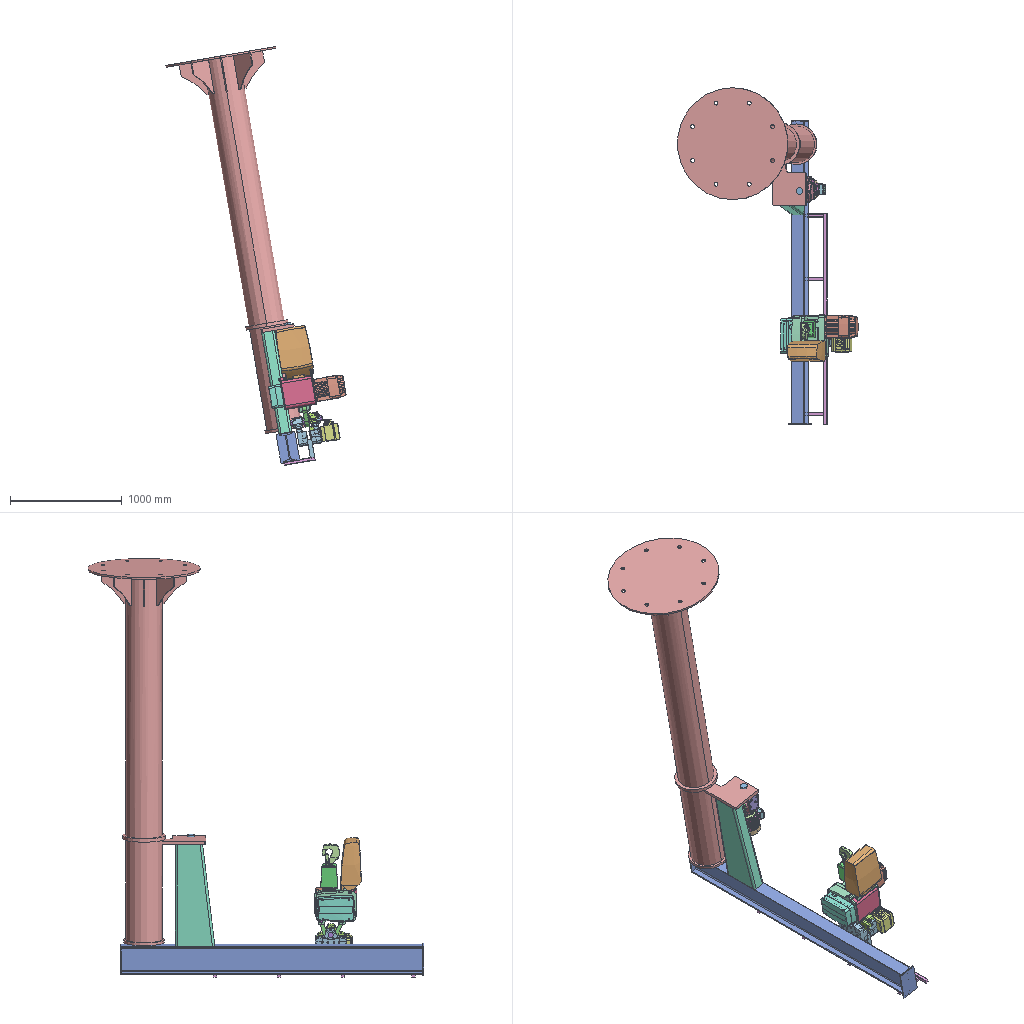Assembly | SolidWorks | 18 different items | 18 placed | box 1611 x 3000 x 3741 mm
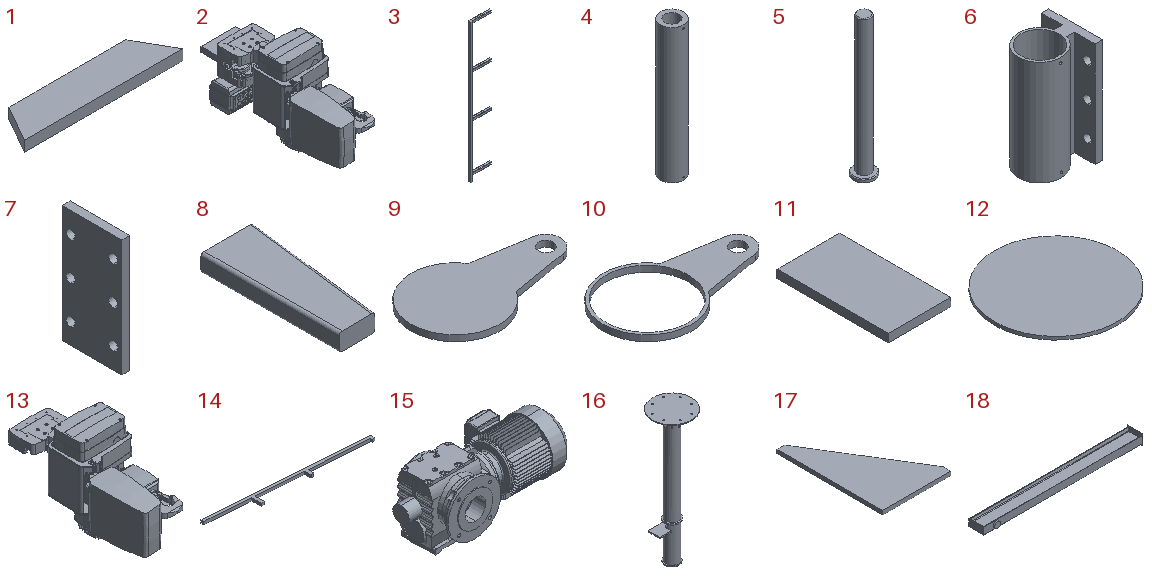Parts list (item | quantity | size | volume | features):
1 | x1 | 152 x 35 x 10 mm | 46200 mm3 | features Extrusion 1
2 | x1 | - | 83796810 mm3 | features BaseBody 21, ICE 3, Scale 1
3 | x1 | 280 x 30 x 1880 mm | 2561715 mm3 | features Extrusion 1, ICE 1
4 | x1 | 80 x 80 x 470 mm | 1439045 mm3 | features Extrusion 1, ICE 1
5 | x1 | 82 x 82 x 541 mm | 1109073 mm3 | features Chamfer 1, Extrusion 1, ICE 1
6 | x1 | 120 x 112 x 220 mm | 732141 mm3 | features ICE 2, Extrusion 1
7 | x1 | 15 x 112 x 220 mm | 349172 mm3 | features ICE 3, Extrusion 1
8 | x1 | 350 x 923 x 118 mm | 31811585 mm3 | features Extrusion 1, Fillet 1
9 | x1 | 496.5 x 293 x 20 mm | 1799574 mm3 | features Extrusion 1
10 | x1 | 496.5 x 293 x 20 mm | 628876 mm3 | features Extrusion 1
11 | x1 | 152 x 270 x 20 mm | 820800 mm3 | features Extrusion 1
12 | x1 | 760 x 760 x 20 mm | 9072920 mm3 | features Extrusion 1
13 | x1 | 284.321 x 725.83 x 459.6 mm | 19917638 mm3 | features BaseBody 17, Scale 1
14 | x1 | 2200 x 220 x 40 mm | 3909881 mm3 | features Extrusion 1
15 | x1 | 558 x 283.5 x 240 mm | 14328030 mm3 | features BaseBody 18, ICE 2
16 | x1 | 1050 x 1000 x 3392 mm | 86673581 mm3 | features ICE 6, CirPattern 1, Extrusion 1
17 | x1 | 180 x 280 x 10 mm | 296000 mm3 | features Extrusion 1
18 | x1 | 2710 x 284 x 170 mm | 14871084 mm3 | features ICE 3, Fillet 2, Extrusion 1
Mates (type | each side: item.copy, entity, surface, feature):
Concentric | 16.1 face cylinder Boss-Extrude1 | 18.1 face cylinder Boss-Extrude3
Coincident | 16.1 face plane Boss-Extrude5 | 18.1 face plane Boss-Extrude3
Parallel | 18.1 face plane Boss-Extrude2 | assembly plane
DistanceDim | 2.1 vertex | 16.1 face plane Boss-Extrude3
Coincident | 18.1 face plane Base | 3.1 face plane Boss-Extrude2 | 2 times
Coincident | 18.1 face plane Boss-Extrude2 | 3.1 face plane Boss-Extrude1
Coincident | 2.1 face plane Boss-Extrude1 | 3.1 face plane Boss-Extrude1
Parallel | 16.1 face plane Boss-Extrude6 | 18.1 face plane Base
Coincident | 16.1 face plane Boss-Extrude6 | 8.1 face plane Boss-Extrude1
Coincident | 18.1 face plane Base | 8.1 face plane Boss-Extrude1
Coincident | 8.1 face plane Boss-Extrude1 | 15.1 face plane Input 19
Coincident | 16.1 face plane Boss-Extrude6 | 15.1 face plane Input 9